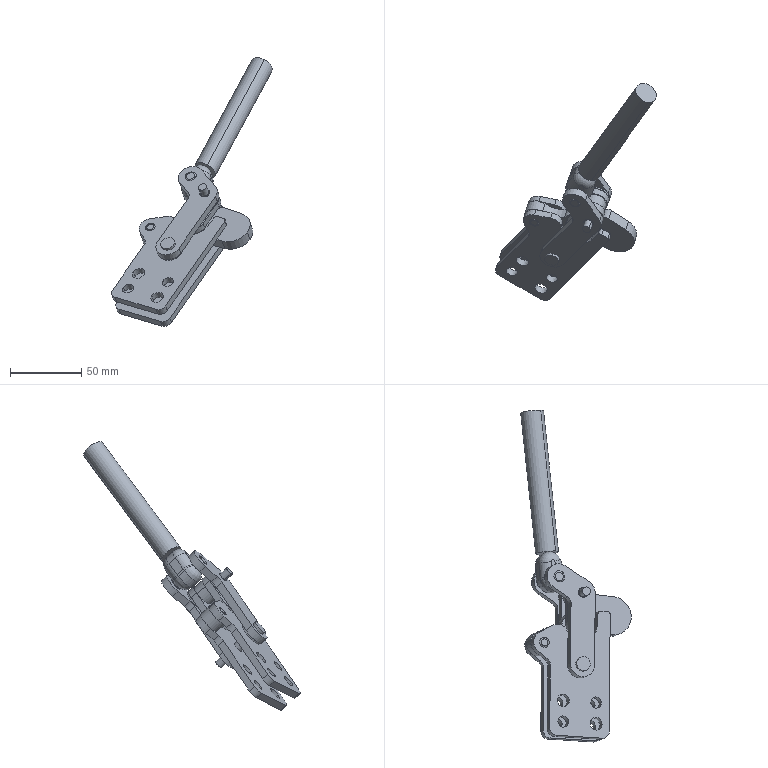Part | SolidWorks | features CompositeCurve 3 | 13 solids | 232 faces | box 112.747 x 151.76 x 188.204 mm | volume 98707 mm3 | cylinder 136 | plane 72 | torus 18 | spline 6 | commonest cylinder face diameters 7 x44 8 x17 17 x9 9 x8 10 x8 16 x7